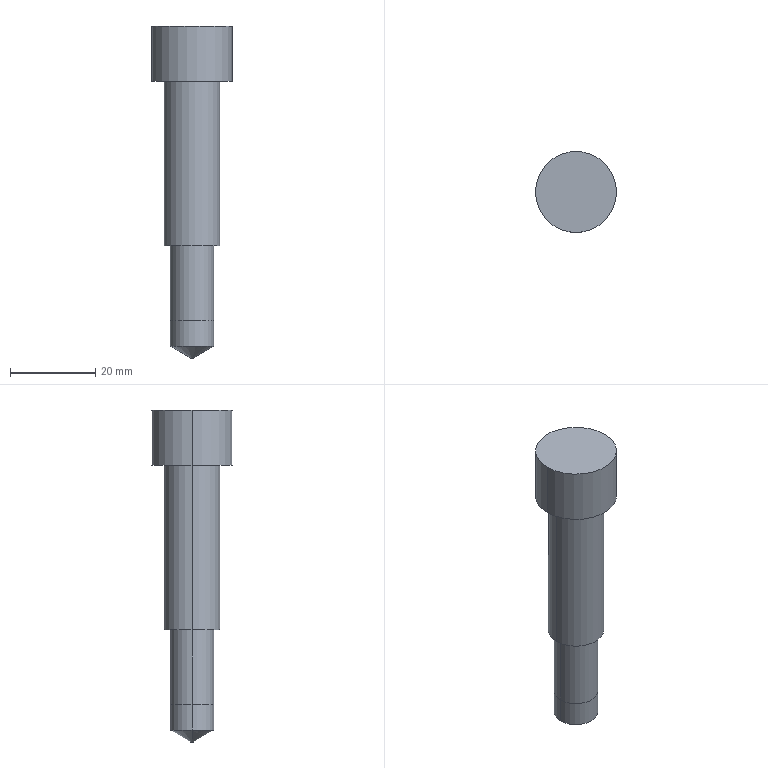Part | Creo | 1 solid | 14 faces | box 19 x 19 x 77.804 mm | volume 10796 mm3 | cylinder 8 | plane 4 | cone 2 | commonest cylinder face diameters 10.199 x2 10.2 x2 13 x2 19 x2
STEP:
#1=CARTESIAN_POINT('',(70.1,75.,91.5));
#2=VERTEX_POINT('',#1);
#3=CARTESIAN_POINT('',(59.9,75.,91.5));
#4=VERTEX_POINT('',#3);
#5=CARTESIAN_POINT('',(65.,75.,91.5));
#6=DIRECTION('',(0.,0.,1.));
#7=DIRECTION('',(1.,0.,0.));
#8=AXIS2_PLACEMENT_3D('',#5,#6,#7);
#9=CIRCLE('',#8,5.1);
#10=EDGE_CURVE('',#2,#4,#9,.T.);
#11=ORIENTED_EDGE('',*,*,#10,.F.);
#12=CARTESIAN_POINT('',(70.1,75.,109.));
#13=VERTEX_POINT('',#12);
#14=CARTESIAN_POINT('',(70.1,75.,91.5));
#15=DIRECTION('',(0.00001429,0.,1.));
#16=VECTOR('',#15,17.5);
#17=LINE('',#14,#16);
#18=EDGE_CURVE('',#2,#13,#17,.T.);
#19=ORIENTED_EDGE('',*,*,#18,.T.);
#20=CARTESIAN_POINT('',(59.9,75.,109.));
#21=VERTEX_POINT('',#20);
#22=CARTESIAN_POINT('',(65.,75.,109.));
#23=DIRECTION('',(0.,0.,1.));
#24=DIRECTION('',(1.,0.,0.));
#25=AXIS2_PLACEMENT_3D('',#22,#23,#24);
#26=CIRCLE('',#25,5.1);
#27=EDGE_CURVE('',#13,#21,#26,.T.);
#28=ORIENTED_EDGE('',*,*,#27,.T.);
#29=CARTESIAN_POINT('',(59.9,75.,91.5));
#30=DIRECTION('',(-0.00001429,0.,1.));
#31=VECTOR('',#30,17.5);
#32=LINE('',#29,#31);
#33=EDGE_CURVE('',#4,#21,#32,.T.);
#34=ORIENTED_EDGE('',*,*,#33,.F.);
#35=EDGE_LOOP('',(#11,#19,#28,#34));
#36=FACE_OUTER_BOUND('',#35,.F.);
#37=CARTESIAN_POINT('',(65.,75.,91.5));
#38=DIRECTION('',(0.,0.,1.));
#39=DIRECTION('',(1.,0.,0.));
#40=AXIS2_PLACEMENT_3D('',#37,#38,#39);
#41=CYLINDRICAL_SURFACE('',#40,5.1);
#42=ADVANCED_FACE('',(#36),#41,.T.);
#43=CARTESIAN_POINT('',(59.901,75.,85.5));
#44=VERTEX_POINT('',#43);
#45=CARTESIAN_POINT('',(70.1,75.,85.5));
#46=VERTEX_POINT('',#45);
#47=CARTESIAN_POINT('',(65.,75.,85.5));
#48=DIRECTION('',(0.,0.,-1.));
#49=DIRECTION('',(-1.,0.,0.));
#50=AXIS2_PLACEMENT_3D('',#47,#48,#49);
#51=CIRCLE('',#50,5.099);
#52=EDGE_CURVE('',#44,#46,#51,.T.);
#53=ORIENTED_EDGE('',*,*,#52,.T.);
#54=CARTESIAN_POINT('',(70.1,75.,91.5));
#55=DIRECTION('',(-0.00004167,0.,-1.));
#56=VECTOR('',#55,6.);
#57=LINE('',#54,#56);
#58=EDGE_CURVE('',#2,#46,#57,.T.);
#59=ORIENTED_EDGE('',*,*,#58,.F.);
#60=ORIENTED_EDGE('',*,*,#10,.T.);
#61=CARTESIAN_POINT('',(59.9,75.,91.5));
#62=DIRECTION('',(0.00004167,0.,-1.));
#63=VECTOR('',#62,6.);
#64=LINE('',#61,#63);
#65=EDGE_CURVE('',#4,#44,#64,.T.);
#66=ORIENTED_EDGE('',*,*,#65,.T.);
#67=EDGE_LOOP('',(#53,#59,#60,#66));
#68=FACE_OUTER_BOUND('',#67,.F.);
#69=CARTESIAN_POINT('',(65.,75.,91.5));
#70=DIRECTION('',(0.,0.,-1.));
#71=DIRECTION('',(-1.,0.,0.));
#72=AXIS2_PLACEMENT_3D('',#69,#70,#71);
#73=CYLINDRICAL_SURFACE('',#72,5.099);
#74=ADVANCED_FACE('',(#68),#73,.T.);
#75=CARTESIAN_POINT('',(64.757,75.,82.696));
#76=VERTEX_POINT('',#75);
#77=CARTESIAN_POINT('',(65.243,75.,82.696));
#78=VERTEX_POINT('',#77);
#79=CARTESIAN_POINT('',(65.,75.,82.696));
#80=DIRECTION('',(0.,0.,-1.));
#81=DIRECTION('',(-1.,0.,0.));
#82=AXIS2_PLACEMENT_3D('',#79,#80,#81);
#83=CIRCLE('',#82,0.2432);
#84=EDGE_CURVE('',#76,#78,#83,.T.);
#85=ORIENTED_EDGE('',*,*,#84,.T.);
#86=CARTESIAN_POINT('',(65.243,75.,82.696));
#87=DIRECTION('',(0.866,0.,0.5));
#88=VECTOR('',#87,5.608);
#89=LINE('',#86,#88);
#90=EDGE_CURVE('',#78,#46,#89,.T.);
#91=ORIENTED_EDGE('',*,*,#90,.T.);
#92=ORIENTED_EDGE('',*,*,#52,.F.);
#93=CARTESIAN_POINT('',(64.757,75.,82.696));
#94=DIRECTION('',(-0.866,0.,0.5));
#95=VECTOR('',#94,5.608);
#96=LINE('',#93,#95);
#97=EDGE_CURVE('',#76,#44,#96,.T.);
#98=ORIENTED_EDGE('',*,*,#97,.F.);
#99=EDGE_LOOP('',(#85,#91,#92,#98));
#100=FACE_OUTER_BOUND('',#99,.F.);
#101=CARTESIAN_POINT('',(65.,75.,84.098));
#102=DIRECTION('',(0.,0.,1.));
#103=DIRECTION('',(1.,0.,0.));
#104=AXIS2_PLACEMENT_3D('',#101,#102,#103);
#105=CONICAL_SURFACE('',#104,2.671,60.);
#106=ADVANCED_FACE('',(#100),#105,.T.);
#107=ORIENTED_EDGE('',*,*,#84,.F.);
#108=CARTESIAN_POINT('',(65.,75.,82.696));
#109=DIRECTION('',(0.,0.,-1.));
#110=DIRECTION('',(1.,0.,0.));
#111=AXIS2_PLACEMENT_3D('',#108,#109,#110);
#112=CIRCLE('',#111,0.2432);
#113=EDGE_CURVE('',#78,#76,#112,.T.);
#114=ORIENTED_EDGE('',*,*,#113,.F.);
#115=EDGE_LOOP('',(#107,#114));
#116=FACE_OUTER_BOUND('',#115,.F.);
#117=CARTESIAN_POINT('',(65.,75.,82.696));
#118=DIRECTION('',(0.,0.,-1.));
#119=DIRECTION('',(-1.,0.,0.));
#120=AXIS2_PLACEMENT_3D('',#117,#118,#119);
#121=PLANE('',#120);
#122=ADVANCED_FACE('',(#116),#121,.T.);
#123=ORIENTED_EDGE('',*,*,#113,.T.);
#124=ORIENTED_EDGE('',*,*,#97,.T.);
#125=CARTESIAN_POINT('',(65.,75.,85.5));
#126=DIRECTION('',(0.,0.,-1.));
#127=DIRECTION('',(1.,0.,0.));
#128=AXIS2_PLACEMENT_3D('',#125,#126,#127);
#129=CIRCLE('',#128,5.099);
#130=EDGE_CURVE('',#46,#44,#129,.T.);
#131=ORIENTED_EDGE('',*,*,#130,.F.);
#132=ORIENTED_EDGE('',*,*,#90,.F.);
#133=EDGE_LOOP('',(#123,#124,#131,#132));
#134=FACE_OUTER_BOUND('',#133,.F.);
#135=CARTESIAN_POINT('',(65.,75.,84.098));
#136=DIRECTION('',(0.,0.,1.));
#137=DIRECTION('',(1.,0.,0.));
#138=AXIS2_PLACEMENT_3D('',#135,#136,#137);
#139=CONICAL_SURFACE('',#138,2.671,60.);
#140=ADVANCED_FACE('',(#134),#139,.T.);
#141=ORIENTED_EDGE('',*,*,#130,.T.);
#142=ORIENTED_EDGE('',*,*,#65,.F.);
#143=CARTESIAN_POINT('',(65.,75.,91.5));
#144=DIRECTION('',(0.,0.,1.));
#145=DIRECTION('',(-1.,0.,0.));
#146=AXIS2_PLACEMENT_3D('',#143,#144,#145);
#147=CIRCLE('',#146,5.1);
#148=EDGE_CURVE('',#4,#2,#147,.T.);
#149=ORIENTED_EDGE('',*,*,#148,.T.);
#150=ORIENTED_EDGE('',*,*,#58,.T.);
#151=EDGE_LOOP('',(#141,#142,#149,#150));
#152=FACE_OUTER_BOUND('',#151,.F.);
#153=CARTESIAN_POINT('',(65.,75.,91.5));
#154=DIRECTION('',(0.,0.,-1.));
#155=DIRECTION('',(-1.,0.,0.));
#156=AXIS2_PLACEMENT_3D('',#153,#154,#155);
#157=CYLINDRICAL_SURFACE('',#156,5.099);
#158=ADVANCED_FACE('',(#152),#157,.T.);
#159=ORIENTED_EDGE('',*,*,#148,.F.);
#160=ORIENTED_EDGE('',*,*,#33,.T.);
#161=CARTESIAN_POINT('',(65.,75.,109.));
#162=DIRECTION('',(0.,0.,1.));
#163=DIRECTION('',(-1.,0.,0.));
#164=AXIS2_PLACEMENT_3D('',#161,#162,#163);
#165=CIRCLE('',#164,5.1);
#166=EDGE_CURVE('',#21,#13,#165,.T.);
#167=ORIENTED_EDGE('',*,*,#166,.T.);
#168=ORIENTED_EDGE('',*,*,#18,.F.);
#169=EDGE_LOOP('',(#159,#160,#167,#168));
#170=FACE_OUTER_BOUND('',#169,.F.);
#171=CARTESIAN_POINT('',(65.,75.,91.5));
#172=DIRECTION('',(0.,0.,1.));
#173=DIRECTION('',(1.,0.,0.));
#174=AXIS2_PLACEMENT_3D('',#171,#172,#173);
#175=CYLINDRICAL_SURFACE('',#174,5.1);
#176=ADVANCED_FACE('',(#170),#175,.T.);
#177=CARTESIAN_POINT('',(71.5,75.,109.));
#178=VERTEX_POINT('',#177);
#179=CARTESIAN_POINT('',(58.5,75.,109.));
#180=VERTEX_POINT('',#179);
#181=CARTESIAN_POINT('',(65.,75.,109.));
#182=DIRECTION('',(0.,0.,-1.));
#183=DIRECTION('',(1.,0.,0.));
#184=AXIS2_PLACEMENT_3D('',#181,#182,#183);
#185=CIRCLE('',#184,6.5);
#186=EDGE_CURVE('',#178,#180,#185,.T.);
#187=ORIENTED_EDGE('',*,*,#186,.F.);
#188=CARTESIAN_POINT('',(65.,75.,109.));
#189=DIRECTION('',(0.,0.,-1.));
#190=DIRECTION('',(-1.,0.,0.));
#191=AXIS2_PLACEMENT_3D('',#188,#189,#190);
#192=CIRCLE('',#191,6.5);
#193=EDGE_CURVE('',#180,#178,#192,.T.);
#194=ORIENTED_EDGE('',*,*,#193,.F.);
#195=EDGE_LOOP('',(#187,#194));
#196=FACE_OUTER_BOUND('',#195,.F.);
#197=ORIENTED_EDGE('',*,*,#166,.F.);
#198=ORIENTED_EDGE('',*,*,#27,.F.);
#199=EDGE_LOOP('',(#197,#198));
#200=FACE_BOUND('',#199,.F.);
#201=CARTESIAN_POINT('',(65.,75.,109.));
#202=DIRECTION('',(0.,0.,-1.));
#203=DIRECTION('',(-1.,0.,0.));
#204=AXIS2_PLACEMENT_3D('',#201,#202,#203);
#205=PLANE('',#204);
#206=ADVANCED_FACE('',(#196,#200),#205,.T.);
#207=CARTESIAN_POINT('',(58.5,75.,147.5));
#208=VERTEX_POINT('',#207);
#209=CARTESIAN_POINT('',(71.5,75.,147.5));
#210=VERTEX_POINT('',#209);
#211=CARTESIAN_POINT('',(65.,75.,147.5));
#212=DIRECTION('',(0.,0.,1.));
#213=DIRECTION('',(-1.,0.,0.));
#214=AXIS2_PLACEMENT_3D('',#211,#212,#213);
#215=CIRCLE('',#214,6.5);
#216=EDGE_CURVE('',#208,#210,#215,.T.);
#217=ORIENTED_EDGE('',*,*,#216,.T.);
#218=CARTESIAN_POINT('',(71.5,75.,109.));
#219=DIRECTION('',(0.,0.,1.));
#220=VECTOR('',#219,38.5);
#221=LINE('',#218,#220);
#222=EDGE_CURVE('',#178,#210,#221,.T.);
#223=ORIENTED_EDGE('',*,*,#222,.F.);
#224=ORIENTED_EDGE('',*,*,#186,.T.);
#225=CARTESIAN_POINT('',(58.5,75.,109.));
#226=DIRECTION('',(0.,0.,1.));
#227=VECTOR('',#226,38.5);
#228=LINE('',#225,#227);
#229=EDGE_CURVE('',#180,#208,#228,.T.);
#230=ORIENTED_EDGE('',*,*,#229,.T.);
#231=EDGE_LOOP('',(#217,#223,#224,#230));
#232=FACE_OUTER_BOUND('',#231,.F.);
#233=CARTESIAN_POINT('',(65.,75.,110.));
#234=DIRECTION('',(0.,0.,1.));
#235=DIRECTION('',(1.,0.,0.));
#236=AXIS2_PLACEMENT_3D('',#233,#234,#235);
#237=CYLINDRICAL_SURFACE('',#236,6.5);
#238=ADVANCED_FACE('',(#232),#237,.T.);
#239=CARTESIAN_POINT('',(74.5,75.,147.5));
#240=VERTEX_POINT('',#239);
#241=CARTESIAN_POINT('',(55.5,75.,147.5));
#242=VERTEX_POINT('',#241);
#243=CARTESIAN_POINT('',(65.,75.,147.5));
#244=DIRECTION('',(0.,0.,-1.));
#245=DIRECTION('',(1.,0.,0.));
#246=AXIS2_PLACEMENT_3D('',#243,#244,#245);
#247=CIRCLE('',#246,9.5);
#248=EDGE_CURVE('',#240,#242,#247,.T.);
#249=ORIENTED_EDGE('',*,*,#248,.F.);
#250=CARTESIAN_POINT('',(65.,75.,147.5));
#251=DIRECTION('',(0.,0.,-1.));
#252=DIRECTION('',(-1.,0.,0.));
#253=AXIS2_PLACEMENT_3D('',#250,#251,#252);
#254=CIRCLE('',#253,9.5);
#255=EDGE_CURVE('',#242,#240,#254,.T.);
#256=ORIENTED_EDGE('',*,*,#255,.F.);
#257=EDGE_LOOP('',(#249,#256));
#258=FACE_OUTER_BOUND('',#257,.F.);
#259=CARTESIAN_POINT('',(65.,75.,147.5));
#260=DIRECTION('',(0.,0.,1.));
#261=DIRECTION('',(1.,0.,0.));
#262=AXIS2_PLACEMENT_3D('',#259,#260,#261);
#263=CIRCLE('',#262,6.5);
#264=EDGE_CURVE('',#210,#208,#263,.T.);
#265=ORIENTED_EDGE('',*,*,#264,.F.);
#266=ORIENTED_EDGE('',*,*,#216,.F.);
#267=EDGE_LOOP('',(#265,#266));
#268=FACE_BOUND('',#267,.F.);
#269=CARTESIAN_POINT('',(65.,75.,147.5));
#270=DIRECTION('',(0.,0.,-1.));
#271=DIRECTION('',(-1.,0.,0.));
#272=AXIS2_PLACEMENT_3D('',#269,#270,#271);
#273=PLANE('',#272);
#274=ADVANCED_FACE('',(#258,#268),#273,.T.);
#275=ORIENTED_EDGE('',*,*,#264,.T.);
#276=ORIENTED_EDGE('',*,*,#229,.F.);
#277=ORIENTED_EDGE('',*,*,#193,.T.);
#278=ORIENTED_EDGE('',*,*,#222,.T.);
#279=EDGE_LOOP('',(#275,#276,#277,#278));
#280=FACE_OUTER_BOUND('',#279,.F.);
#281=CARTESIAN_POINT('',(65.,75.,110.));
#282=DIRECTION('',(0.,0.,1.));
#283=DIRECTION('',(1.,0.,0.));
#284=AXIS2_PLACEMENT_3D('',#281,#282,#283);
#285=CYLINDRICAL_SURFACE('',#284,6.5);
#286=ADVANCED_FACE('',(#280),#285,.T.);
#287=CARTESIAN_POINT('',(55.5,75.,160.5));
#288=VERTEX_POINT('',#287);
#289=CARTESIAN_POINT('',(74.5,75.,160.5));
#290=VERTEX_POINT('',#289);
#291=CARTESIAN_POINT('',(65.,75.,160.5));
#292=DIRECTION('',(0.,0.,1.));
#293=DIRECTION('',(-1.,0.,0.));
#294=AXIS2_PLACEMENT_3D('',#291,#292,#293);
#295=CIRCLE('',#294,9.5);
#296=EDGE_CURVE('',#288,#290,#295,.T.);
#297=ORIENTED_EDGE('',*,*,#296,.T.);
#298=CARTESIAN_POINT('',(74.5,75.,147.5));
#299=DIRECTION('',(0.,0.,1.));
#300=VECTOR('',#299,13.);
#301=LINE('',#298,#300);
#302=EDGE_CURVE('',#240,#290,#301,.T.);
#303=ORIENTED_EDGE('',*,*,#302,.F.);
#304=ORIENTED_EDGE('',*,*,#248,.T.);
#305=CARTESIAN_POINT('',(55.5,75.,147.5));
#306=DIRECTION('',(0.,0.,1.));
#307=VECTOR('',#306,13.);
#308=LINE('',#305,#307);
#309=EDGE_CURVE('',#242,#288,#308,.T.);
#310=ORIENTED_EDGE('',*,*,#309,.T.);
#311=EDGE_LOOP('',(#297,#303,#304,#310));
#312=FACE_OUTER_BOUND('',#311,.F.);
#313=CARTESIAN_POINT('',(65.,75.,147.5));
#314=DIRECTION('',(0.,0.,1.));
#315=DIRECTION('',(1.,0.,0.));
#316=AXIS2_PLACEMENT_3D('',#313,#314,#315);
#317=CYLINDRICAL_SURFACE('',#316,9.5);
#318=ADVANCED_FACE('',(#312),#317,.T.);
#319=CARTESIAN_POINT('',(65.,75.,160.5));
#320=DIRECTION('',(0.,0.,1.));
#321=DIRECTION('',(1.,0.,0.));
#322=AXIS2_PLACEMENT_3D('',#319,#320,#321);
#323=CIRCLE('',#322,9.5);
#324=EDGE_CURVE('',#290,#288,#323,.T.);
#325=ORIENTED_EDGE('',*,*,#324,.F.);
#326=ORIENTED_EDGE('',*,*,#296,.F.);
#327=EDGE_LOOP('',(#325,#326));
#328=FACE_OUTER_BOUND('',#327,.F.);
#329=CARTESIAN_POINT('',(65.,75.,160.5));
#330=DIRECTION('',(0.,0.,1.));
#331=DIRECTION('',(1.,0.,0.));
#332=AXIS2_PLACEMENT_3D('',#329,#330,#331);
#333=PLANE('',#332);
#334=ADVANCED_FACE('',(#328),#333,.T.);
#335=ORIENTED_EDGE('',*,*,#324,.T.);
#336=ORIENTED_EDGE('',*,*,#309,.F.);
#337=ORIENTED_EDGE('',*,*,#255,.T.);
#338=ORIENTED_EDGE('',*,*,#302,.T.);
#339=EDGE_LOOP('',(#335,#336,#337,#338));
#340=FACE_OUTER_BOUND('',#339,.F.);
#341=CARTESIAN_POINT('',(65.,75.,147.5));
#342=DIRECTION('',(0.,0.,1.));
#343=DIRECTION('',(1.,0.,0.));
#344=AXIS2_PLACEMENT_3D('',#341,#342,#343);
#345=CYLINDRICAL_SURFACE('',#344,9.5);
#346=ADVANCED_FACE('',(#340),#345,.T.);
#347=CLOSED_SHELL('',(#42,#74,#106,#122,#140,#158,#176,#206,#238,#274,#286,#318,#334,#346));
#348=MANIFOLD_SOLID_BREP('',#347);
#349=(LENGTH_UNIT()NAMED_UNIT(*)SI_UNIT(.MILLI.,.METRE.));
#350=UNCERTAINTY_MEASURE_WITH_UNIT(LENGTH_MEASURE(0.008231),#349,'','');
#351=(NAMED_UNIT(*)PLANE_ANGLE_UNIT()SI_UNIT($,.RADIAN.));
#352=PLANE_ANGLE_MEASURE_WITH_UNIT(PLANE_ANGLE_MEASURE(0.01745),#351);
#353=(CONVERSION_BASED_UNIT('DEGREE',#352)NAMED_UNIT(*)PLANE_ANGLE_UNIT());
#354=(NAMED_UNIT(*)SI_UNIT($,.STERADIAN.)SOLID_ANGLE_UNIT());
#355=(GEOMETRIC_REPRESENTATION_CONTEXT(3)GLOBAL_UNCERTAINTY_ASSIGNED_CONTEXT((#350))GLOBAL_UNIT_ASSIGNED_CONTEXT((#349,#353,#354))REPRESENTATION_CONTEXT('',''));
#356=ADVANCED_BREP_SHAPE_REPRESENTATION('',(#348),#355);